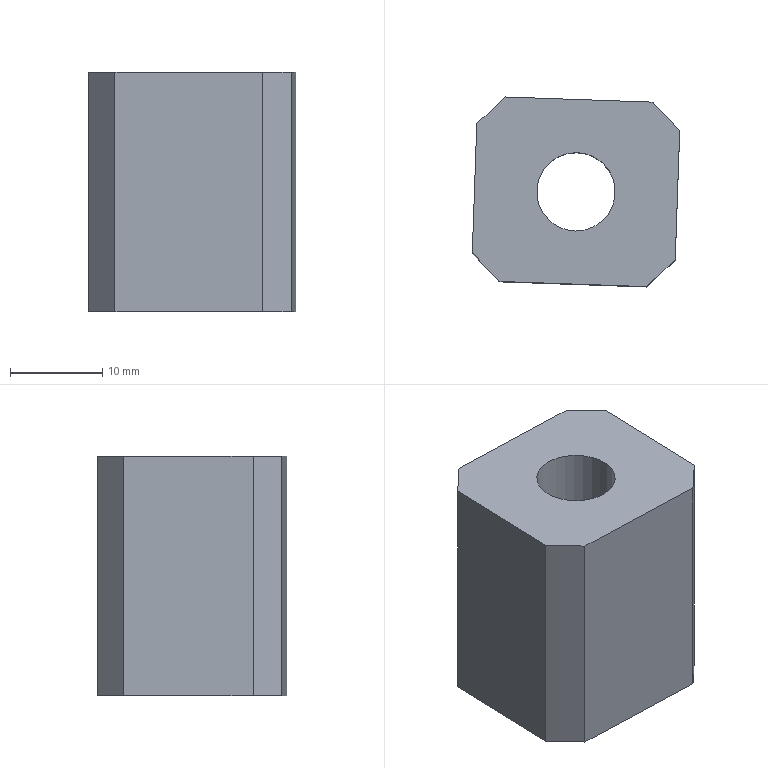Part | NX | features LB-21 2 | 1 solid | 13 faces | box 22.475 x 20.546 x 26 mm | volume 8428 mm3 | plane 11 | cylinder 2 | commonest cylinder face diameters 8.5 x1 14 x1
STEP:
#1=CARTESIAN_POINT('',(3794.927,-985.155,785.216));
#2=VERTEX_POINT('',#1);
#3=CARTESIAN_POINT('',(3810.917,-985.713,785.216));
#4=VERTEX_POINT('',#3);
#5=CARTESIAN_POINT('',(3771.941,-984.352,785.216));
#6=DIRECTION('',(0.9994,-0.0349,0.000000002));
#7=VECTOR('',#6,1000.);
#8=LINE('',#5,#7);
#9=EDGE_CURVE('',#2,#4,#8,.T.);
#10=ORIENTED_EDGE('',*,*,#9,.T.);
#11=CARTESIAN_POINT('',(3810.917,-985.713,811.216));
#12=VERTEX_POINT('',#11);
#13=CARTESIAN_POINT('',(3810.917,-985.713,792.216));
#14=DIRECTION('',(-0.000000002,0.,1.));
#15=VECTOR('',#14,1000.);
#16=LINE('',#13,#15);
#17=EDGE_CURVE('',#4,#12,#16,.T.);
#18=ORIENTED_EDGE('',*,*,#17,.T.);
#19=CARTESIAN_POINT('',(3794.927,-985.155,811.216));
#20=VERTEX_POINT('',#19);
#21=CARTESIAN_POINT('',(3771.941,-984.352,811.216));
#22=DIRECTION('',(0.9994,-0.0349,0.000000002));
#23=VECTOR('',#22,1000.);
#24=LINE('',#21,#23);
#25=EDGE_CURVE('',#20,#12,#24,.T.);
#26=ORIENTED_EDGE('',*,*,#25,.F.);
#27=CARTESIAN_POINT('',(3794.927,-985.155,792.216));
#28=DIRECTION('',(0.000000002,0.,-1.));
#29=VECTOR('',#28,1000.);
#30=LINE('',#27,#29);
#31=EDGE_CURVE('',#20,#2,#30,.T.);
#32=ORIENTED_EDGE('',*,*,#31,.T.);
#33=EDGE_LOOP('',(#10,#18,#26,#32));
#34=FACE_BOUND('',#33,.T.);
#35=CARTESIAN_POINT('',(3771.941,-984.352,792.216));
#36=DIRECTION('',(-0.0349,-0.9994,0.));
#37=DIRECTION('',(0.9994,-0.0349,0.000000002));
#38=AXIS2_PLACEMENT_3D('',#35,#36,#37);
#39=PLANE('',#38);
#40=ADVANCED_FACE('',(#34),#39,.T.);
#41=CARTESIAN_POINT('',(3796.275,-975.196,785.216));
#42=VERTEX_POINT('',#41);
#43=CARTESIAN_POINT('',(3803.271,-975.44,785.216));
#44=DIRECTION('',(-0.000000002,0.,1.));
#45=DIRECTION('',(-0.9994,0.0349,-0.000000002));
#46=AXIS2_PLACEMENT_3D('',#43,#44,#45);
#47=CIRCLE('',#46,7.);
#48=EDGE_CURVE('',#42,#42,#47,.T.);
#49=ORIENTED_EDGE('',*,*,#48,.T.);
#50=EDGE_LOOP('',(#49));
#51=FACE_BOUND('',#50,.T.);
#52=CARTESIAN_POINT('',(3792.033,-982.052,785.216));
#53=VERTEX_POINT('',#52);
#54=CARTESIAN_POINT('',(3792.522,-968.06,785.216));
#55=VERTEX_POINT('',#54);
#56=CARTESIAN_POINT('',(3792.557,-967.061,785.216));
#57=DIRECTION('',(0.0349,0.9994,0.));
#58=VECTOR('',#57,1000.);
#59=LINE('',#56,#58);
#60=EDGE_CURVE('',#53,#55,#59,.T.);
#61=ORIENTED_EDGE('',*,*,#60,.T.);
#62=CARTESIAN_POINT('',(3795.625,-965.167,785.216));
#63=VERTEX_POINT('',#62);
#64=CARTESIAN_POINT('',(3782.179,-977.705,785.216));
#65=DIRECTION('',(0.7314,0.682,0.000000001));
#66=VECTOR('',#65,1000.);
#67=LINE('',#64,#66);
#68=EDGE_CURVE('',#55,#63,#67,.T.);
#69=ORIENTED_EDGE('',*,*,#68,.T.);
#70=CARTESIAN_POINT('',(3811.615,-965.725,785.216));
#71=VERTEX_POINT('',#70);
#72=CARTESIAN_POINT('',(3772.639,-964.364,785.216));
#73=DIRECTION('',(0.9994,-0.0349,0.000000002));
#74=VECTOR('',#73,1000.);
#75=LINE('',#72,#74);
#76=EDGE_CURVE('',#63,#71,#75,.T.);
#77=ORIENTED_EDGE('',*,*,#76,.T.);
#78=CARTESIAN_POINT('',(3814.508,-968.828,785.216));
#79=VERTEX_POINT('',#78);
#80=CARTESIAN_POINT('',(3794.254,-947.108,785.216));
#81=DIRECTION('',(0.682,-0.7314,0.000000001));
#82=VECTOR('',#81,1000.);
#83=LINE('',#80,#82);
#84=EDGE_CURVE('',#71,#79,#83,.T.);
#85=ORIENTED_EDGE('',*,*,#84,.T.);
#86=CARTESIAN_POINT('',(3814.02,-982.819,785.216));
#87=VERTEX_POINT('',#86);
#88=CARTESIAN_POINT('',(3814.543,-967.829,785.216));
#89=DIRECTION('',(-0.0349,-0.9994,0.));
#90=VECTOR('',#89,1000.);
#91=LINE('',#88,#90);
#92=EDGE_CURVE('',#79,#87,#91,.T.);
#93=ORIENTED_EDGE('',*,*,#92,.T.);
#94=CARTESIAN_POINT('',(3800.574,-995.358,785.216));
#95=DIRECTION('',(-0.7314,-0.682,-0.000000001));
#96=VECTOR('',#95,1000.);
#97=LINE('',#94,#96);
#98=EDGE_CURVE('',#87,#4,#97,.T.);
#99=ORIENTED_EDGE('',*,*,#98,.T.);
#100=ORIENTED_EDGE('',*,*,#9,.F.);
#101=CARTESIAN_POINT('',(3774.672,-963.435,785.216));
#102=DIRECTION('',(-0.682,0.7314,-0.000000001));
#103=VECTOR('',#102,1000.);
#104=LINE('',#101,#103);
#105=EDGE_CURVE('',#2,#53,#104,.T.);
#106=ORIENTED_EDGE('',*,*,#105,.T.);
#107=EDGE_LOOP('',(#61,#69,#77,#85,#93,#99,#100,#106));
#108=FACE_BOUND('',#107,.T.);
#109=CARTESIAN_POINT('',(3772.569,-966.363,785.216));
#110=DIRECTION('',(0.000000002,0.,-1.));
#111=DIRECTION('',(-0.9994,0.0349,-0.000000002));
#112=AXIS2_PLACEMENT_3D('',#109,#110,#111);
#113=PLANE('',#112);
#114=ADVANCED_FACE('',(#51,#108),#113,.T.);
#115=CARTESIAN_POINT('',(3806.744,-977.889,811.216));
#116=VERTEX_POINT('',#115);
#117=CARTESIAN_POINT('',(3803.271,-975.44,811.216));
#118=DIRECTION('',(0.000000002,0.,-1.));
#119=DIRECTION('',(0.8173,-0.5762,0.000000002));
#120=AXIS2_PLACEMENT_3D('',#117,#118,#119);
#121=CIRCLE('',#120,4.25);
#122=EDGE_CURVE('',#116,#116,#121,.T.);
#123=ORIENTED_EDGE('',*,*,#122,.T.);
#124=EDGE_LOOP('',(#123));
#125=FACE_BOUND('',#124,.T.);
#126=CARTESIAN_POINT('',(3811.615,-965.725,811.216));
#127=VERTEX_POINT('',#126);
#128=CARTESIAN_POINT('',(3795.625,-965.167,811.216));
#129=VERTEX_POINT('',#128);
#130=CARTESIAN_POINT('',(3772.639,-964.364,811.216));
#131=DIRECTION('',(-0.9994,0.0349,-0.000000002));
#132=VECTOR('',#131,1000.);
#133=LINE('',#130,#132);
#134=EDGE_CURVE('',#127,#129,#133,.T.);
#135=ORIENTED_EDGE('',*,*,#134,.T.);
#136=CARTESIAN_POINT('',(3792.522,-968.06,811.216));
#137=VERTEX_POINT('',#136);
#138=CARTESIAN_POINT('',(3782.179,-977.705,811.216));
#139=DIRECTION('',(-0.7314,-0.682,-0.000000001));
#140=VECTOR('',#139,1000.);
#141=LINE('',#138,#140);
#142=EDGE_CURVE('',#129,#137,#141,.T.);
#143=ORIENTED_EDGE('',*,*,#142,.T.);
#144=CARTESIAN_POINT('',(3792.033,-982.052,811.216));
#145=VERTEX_POINT('',#144);
#146=CARTESIAN_POINT('',(3792.557,-967.061,811.216));
#147=DIRECTION('',(-0.0349,-0.9994,0.));
#148=VECTOR('',#147,1000.);
#149=LINE('',#146,#148);
#150=EDGE_CURVE('',#137,#145,#149,.T.);
#151=ORIENTED_EDGE('',*,*,#150,.T.);
#152=CARTESIAN_POINT('',(3774.672,-963.435,811.216));
#153=DIRECTION('',(0.682,-0.7314,0.000000001));
#154=VECTOR('',#153,1000.);
#155=LINE('',#152,#154);
#156=EDGE_CURVE('',#145,#20,#155,.T.);
#157=ORIENTED_EDGE('',*,*,#156,.T.);
#158=ORIENTED_EDGE('',*,*,#25,.T.);
#159=CARTESIAN_POINT('',(3814.02,-982.819,811.216));
#160=VERTEX_POINT('',#159);
#161=CARTESIAN_POINT('',(3800.574,-995.358,811.216));
#162=DIRECTION('',(0.7314,0.682,0.000000001));
#163=VECTOR('',#162,1000.);
#164=LINE('',#161,#163);
#165=EDGE_CURVE('',#12,#160,#164,.T.);
#166=ORIENTED_EDGE('',*,*,#165,.T.);
#167=CARTESIAN_POINT('',(3814.508,-968.828,811.216));
#168=VERTEX_POINT('',#167);
#169=CARTESIAN_POINT('',(3814.543,-967.829,811.216));
#170=DIRECTION('',(0.0349,0.9994,0.));
#171=VECTOR('',#170,1000.);
#172=LINE('',#169,#171);
#173=EDGE_CURVE('',#160,#168,#172,.T.);
#174=ORIENTED_EDGE('',*,*,#173,.T.);
#175=CARTESIAN_POINT('',(3794.254,-947.108,811.216));
#176=DIRECTION('',(-0.682,0.7314,-0.000000001));
#177=VECTOR('',#176,1000.);
#178=LINE('',#175,#177);
#179=EDGE_CURVE('',#168,#127,#178,.T.);
#180=ORIENTED_EDGE('',*,*,#179,.T.);
#181=EDGE_LOOP('',(#135,#143,#151,#157,#158,#166,#174,#180));
#182=FACE_BOUND('',#181,.T.);
#183=CARTESIAN_POINT('',(3772.569,-966.363,811.216));
#184=DIRECTION('',(-0.000000002,0.,1.));
#185=DIRECTION('',(0.9994,-0.0349,0.000000002));
#186=AXIS2_PLACEMENT_3D('',#183,#184,#185);
#187=PLANE('',#186);
#188=ADVANCED_FACE('',(#125,#182),#187,.T.);
#189=CARTESIAN_POINT('',(3806.744,-977.889,796.216));
#190=VERTEX_POINT('',#189);
#191=CARTESIAN_POINT('',(3803.271,-975.44,796.216));
#192=DIRECTION('',(0.000000002,0.,-1.));
#193=DIRECTION('',(0.8173,-0.5762,0.000000002));
#194=AXIS2_PLACEMENT_3D('',#191,#192,#193);
#195=CIRCLE('',#194,4.25);
#196=EDGE_CURVE('',#190,#190,#195,.T.);
#197=ORIENTED_EDGE('',*,*,#196,.T.);
#198=EDGE_LOOP('',(#197));
#199=FACE_BOUND('',#198,.T.);
#200=ORIENTED_EDGE('',*,*,#122,.F.);
#201=EDGE_LOOP('',(#200));
#202=FACE_BOUND('',#201,.T.);
#203=CARTESIAN_POINT('',(3803.271,-975.44,803.216));
#204=DIRECTION('',(0.000000002,0.,-1.));
#205=DIRECTION('',(-0.9994,0.0349,-0.000000002));
#206=AXIS2_PLACEMENT_3D('',#203,#204,#205);
#207=CYLINDRICAL_SURFACE('',#206,4.25);
#208=ADVANCED_FACE('',(#199,#202),#207,.F.);
#209=ORIENTED_EDGE('',*,*,#196,.F.);
#210=EDGE_LOOP('',(#209));
#211=FACE_BOUND('',#210,.T.);
#212=CARTESIAN_POINT('',(3810.267,-975.684,796.216));
#213=VERTEX_POINT('',#212);
#214=CARTESIAN_POINT('',(3803.271,-975.44,796.216));
#215=DIRECTION('',(0.000000002,0.,-1.));
#216=DIRECTION('',(0.9994,-0.0349,0.000000002));
#217=AXIS2_PLACEMENT_3D('',#214,#215,#216);
#218=CIRCLE('',#217,7.);
#219=EDGE_CURVE('',#213,#213,#218,.T.);
#220=ORIENTED_EDGE('',*,*,#219,.T.);
#221=EDGE_LOOP('',(#220));
#222=FACE_BOUND('',#221,.T.);
#223=CARTESIAN_POINT('',(3803.271,-975.44,796.216));
#224=DIRECTION('',(-0.000000002,0.,1.));
#225=DIRECTION('',(0.9994,-0.0349,0.000000002));
#226=AXIS2_PLACEMENT_3D('',#223,#224,#225);
#227=PLANE('',#226);
#228=ADVANCED_FACE('',(#211,#222),#227,.F.);
#229=ORIENTED_EDGE('',*,*,#48,.F.);
#230=EDGE_LOOP('',(#229));
#231=FACE_BOUND('',#230,.T.);
#232=ORIENTED_EDGE('',*,*,#219,.F.);
#233=EDGE_LOOP('',(#232));
#234=FACE_BOUND('',#233,.T.);
#235=CARTESIAN_POINT('',(3803.271,-975.44,796.216));
#236=DIRECTION('',(0.000000002,0.,-1.));
#237=DIRECTION('',(-0.9994,0.0349,-0.000000002));
#238=AXIS2_PLACEMENT_3D('',#235,#236,#237);
#239=CYLINDRICAL_SURFACE('',#238,7.);
#240=ADVANCED_FACE('',(#231,#234),#239,.F.);
#241=ORIENTED_EDGE('',*,*,#92,.F.);
#242=CARTESIAN_POINT('',(3814.508,-968.828,795.216));
#243=DIRECTION('',(-0.000000002,0.,1.));
#244=VECTOR('',#243,1000.);
#245=LINE('',#242,#244);
#246=EDGE_CURVE('',#79,#168,#245,.T.);
#247=ORIENTED_EDGE('',*,*,#246,.T.);
#248=ORIENTED_EDGE('',*,*,#173,.F.);
#249=CARTESIAN_POINT('',(3814.02,-982.819,795.216));
#250=DIRECTION('',(0.000000002,0.,-1.));
#251=VECTOR('',#250,1000.);
#252=LINE('',#249,#251);
#253=EDGE_CURVE('',#160,#87,#252,.T.);
#254=ORIENTED_EDGE('',*,*,#253,.T.);
#255=EDGE_LOOP('',(#241,#247,#248,#254));
#256=FACE_BOUND('',#255,.T.);
#257=CARTESIAN_POINT('',(3814.264,-975.824,795.216));
#258=DIRECTION('',(0.9994,-0.0349,0.000000002));
#259=DIRECTION('',(-0.000000002,0.,1.));
#260=AXIS2_PLACEMENT_3D('',#257,#258,#259);
#261=PLANE('',#260);
#262=ADVANCED_FACE('',(#256),#261,.T.);
#263=ORIENTED_EDGE('',*,*,#76,.F.);
#264=CARTESIAN_POINT('',(3795.625,-965.167,795.216));
#265=DIRECTION('',(-0.000000002,0.,1.));
#266=VECTOR('',#265,1000.);
#267=LINE('',#264,#266);
#268=EDGE_CURVE('',#63,#129,#267,.T.);
#269=ORIENTED_EDGE('',*,*,#268,.T.);
#270=ORIENTED_EDGE('',*,*,#134,.F.);
#271=CARTESIAN_POINT('',(3811.615,-965.725,795.216));
#272=DIRECTION('',(0.000000002,0.,-1.));
#273=VECTOR('',#272,1000.);
#274=LINE('',#271,#273);
#275=EDGE_CURVE('',#127,#71,#274,.T.);
#276=ORIENTED_EDGE('',*,*,#275,.T.);
#277=EDGE_LOOP('',(#263,#269,#270,#276));
#278=FACE_BOUND('',#277,.T.);
#279=CARTESIAN_POINT('',(3793.626,-965.097,795.216));
#280=DIRECTION('',(0.0349,0.9994,0.));
#281=DIRECTION('',(-0.9994,0.0349,-0.000000002));
#282=AXIS2_PLACEMENT_3D('',#279,#280,#281);
#283=PLANE('',#282);
#284=ADVANCED_FACE('',(#278),#283,.T.);
#285=ORIENTED_EDGE('',*,*,#150,.F.);
#286=CARTESIAN_POINT('',(3792.522,-968.06,795.216));
#287=DIRECTION('',(0.000000002,0.,-1.));
#288=VECTOR('',#287,1000.);
#289=LINE('',#286,#288);
#290=EDGE_CURVE('',#137,#55,#289,.T.);
#291=ORIENTED_EDGE('',*,*,#290,.T.);
#292=ORIENTED_EDGE('',*,*,#60,.F.);
#293=CARTESIAN_POINT('',(3792.033,-982.052,795.216));
#294=DIRECTION('',(-0.000000002,0.,1.));
#295=VECTOR('',#294,1000.);
#296=LINE('',#293,#295);
#297=EDGE_CURVE('',#53,#145,#296,.T.);
#298=ORIENTED_EDGE('',*,*,#297,.T.);
#299=EDGE_LOOP('',(#285,#291,#292,#298));
#300=FACE_BOUND('',#299,.T.);
#301=CARTESIAN_POINT('',(3792.278,-975.056,795.216));
#302=DIRECTION('',(-0.9994,0.0349,-0.000000002));
#303=DIRECTION('',(0.000000002,0.,-1.));
#304=AXIS2_PLACEMENT_3D('',#301,#302,#303);
#305=PLANE('',#304);
#306=ADVANCED_FACE('',(#300),#305,.T.);
#307=ORIENTED_EDGE('',*,*,#68,.F.);
#308=ORIENTED_EDGE('',*,*,#290,.F.);
#309=ORIENTED_EDGE('',*,*,#142,.F.);
#310=ORIENTED_EDGE('',*,*,#268,.F.);
#311=EDGE_LOOP('',(#307,#308,#309,#310));
#312=FACE_BOUND('',#311,.T.);
#313=CARTESIAN_POINT('',(3795.625,-965.167,795.216));
#314=DIRECTION('',(0.682,-0.7314,0.000000001));
#315=DIRECTION('',(-0.7314,-0.682,-0.000000001));
#316=AXIS2_PLACEMENT_3D('',#313,#314,#315);
#317=PLANE('',#316);
#318=ADVANCED_FACE('',(#312),#317,.F.);
#319=ORIENTED_EDGE('',*,*,#179,.F.);
#320=ORIENTED_EDGE('',*,*,#246,.F.);
#321=ORIENTED_EDGE('',*,*,#84,.F.);
#322=ORIENTED_EDGE('',*,*,#275,.F.);
#323=EDGE_LOOP('',(#319,#320,#321,#322));
#324=FACE_BOUND('',#323,.T.);
#325=CARTESIAN_POINT('',(3811.615,-965.725,795.216));
#326=DIRECTION('',(-0.7314,-0.682,-0.000000001));
#327=DIRECTION('',(-0.682,0.7314,-0.000000001));
#328=AXIS2_PLACEMENT_3D('',#325,#326,#327);
#329=PLANE('',#328);
#330=ADVANCED_FACE('',(#324),#329,.F.);
#331=ORIENTED_EDGE('',*,*,#98,.F.);
#332=ORIENTED_EDGE('',*,*,#253,.F.);
#333=ORIENTED_EDGE('',*,*,#165,.F.);
#334=ORIENTED_EDGE('',*,*,#17,.F.);
#335=EDGE_LOOP('',(#331,#332,#333,#334));
#336=FACE_BOUND('',#335,.T.);
#337=CARTESIAN_POINT('',(3810.917,-985.713,792.216));
#338=DIRECTION('',(-0.682,0.7314,-0.000000001));
#339=DIRECTION('',(0.7314,0.682,0.000000001));
#340=AXIS2_PLACEMENT_3D('',#337,#338,#339);
#341=PLANE('',#340);
#342=ADVANCED_FACE('',(#336),#341,.F.);
#343=ORIENTED_EDGE('',*,*,#156,.F.);
#344=ORIENTED_EDGE('',*,*,#297,.F.);
#345=ORIENTED_EDGE('',*,*,#105,.F.);
#346=ORIENTED_EDGE('',*,*,#31,.F.);
#347=EDGE_LOOP('',(#343,#344,#345,#346));
#348=FACE_BOUND('',#347,.T.);
#349=CARTESIAN_POINT('',(3794.927,-985.155,792.216));
#350=DIRECTION('',(0.7314,0.682,0.000000001));
#351=DIRECTION('',(0.682,-0.7314,0.000000001));
#352=AXIS2_PLACEMENT_3D('',#349,#350,#351);
#353=PLANE('',#352);
#354=ADVANCED_FACE('',(#348),#353,.F.);
#355=CLOSED_SHELL('',(#40,#114,#188,#208,#228,#240,#262,#284,#306,#318,#330,#342,#354));
#356=MANIFOLD_SOLID_BREP('',#355);
#357=(LENGTH_UNIT()NAMED_UNIT(*)SI_UNIT(.MILLI.,.METRE.));
#358=UNCERTAINTY_MEASURE_WITH_UNIT(LENGTH_MEASURE(0.00001),#357,'','');
#359=(NAMED_UNIT(*)PLANE_ANGLE_UNIT()SI_UNIT($,.RADIAN.));
#360=(NAMED_UNIT(*)SI_UNIT($,.STERADIAN.)SOLID_ANGLE_UNIT());
#361=(GEOMETRIC_REPRESENTATION_CONTEXT(3)GLOBAL_UNCERTAINTY_ASSIGNED_CONTEXT((#358))GLOBAL_UNIT_ASSIGNED_CONTEXT((#357,#359,#360))REPRESENTATION_CONTEXT('',''));
#362=ADVANCED_BREP_SHAPE_REPRESENTATION('',(#356),#361);